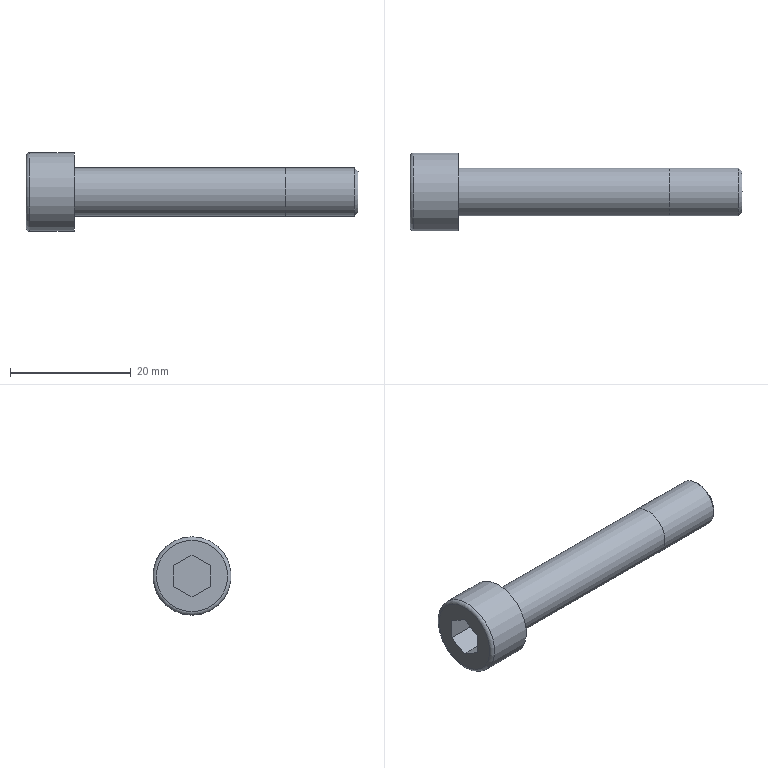Part | STEP file | solid 2 | 1 solid | 21 faces | box 55 x 13 x 13 mm | volume 3119 mm3 | plane 14 | cylinder 5 | torus 1 | cone 1 | commonest cylinder face diameters 6.8 x1 6.98 x1 7.99 x1 8 x1 13 x1